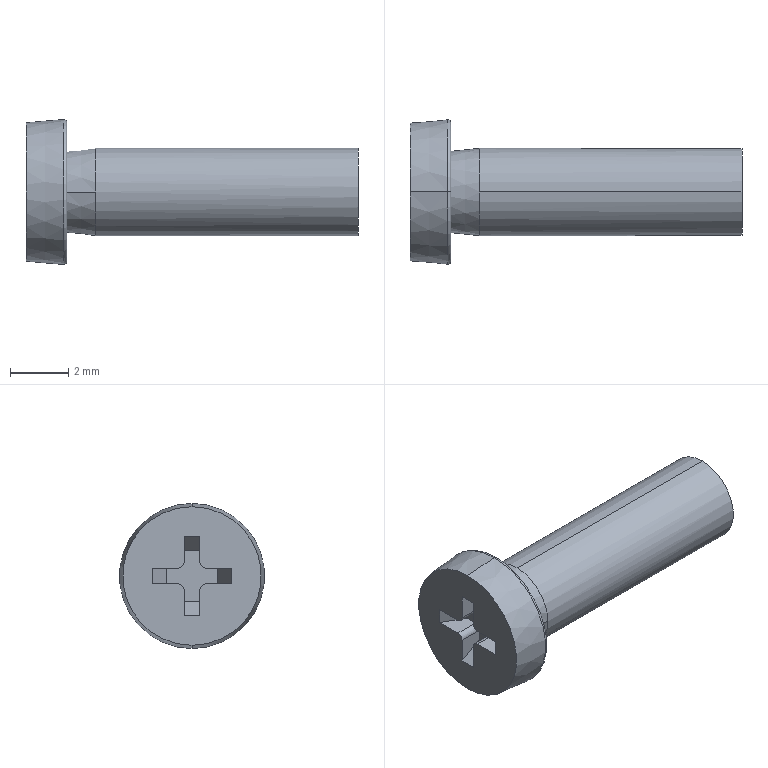Part | SolidWorks | features Draft 2, Fillet 2, Boss 1, Cut 1, Extrusion 1, LPattern 1, PLine 1, RevCut 1 | 1 solid | 28 faces | box 11.4 x 4.982 x 4.982 mm | volume 94.532 mm3 | plane 16 | cylinder 6 | cone 4 | torus 2 | commonest cylinder face diameters 0.4 x4 3 x2
STEP:
#1=CARTESIAN_POINT('',(1.291,0.,2.49));
#2=VERTEX_POINT('',#1);
#3=CARTESIAN_POINT('',(1.291,0.,-2.49));
#4=VERTEX_POINT('',#3);
#5=CARTESIAN_POINT('',(1.291,0.,0.));
#6=DIRECTION('',(-1.,0.,0.));
#7=DIRECTION('',(0.,0.,1.));
#8=AXIS2_PLACEMENT_3D('',#5,#6,#7);
#9=CIRCLE('',#8,2.49);
#10=EDGE_CURVE('',#2,#4,#9,.T.);
#11=ORIENTED_EDGE('',*,*,#10,.F.);
#12=CARTESIAN_POINT('',(1.4,0.,2.391));
#13=VERTEX_POINT('',#12);
#14=CARTESIAN_POINT('',(1.3,0.,2.391));
#15=DIRECTION('',(0.,1.,0.));
#16=DIRECTION('',(0.,0.,1.));
#17=AXIS2_PLACEMENT_3D('',#14,#15,#16);
#18=CIRCLE('',#17,0.1);
#19=EDGE_CURVE('',#2,#13,#18,.T.);
#20=ORIENTED_EDGE('',*,*,#19,.T.);
#21=CARTESIAN_POINT('',(1.4,0.,-2.391));
#22=VERTEX_POINT('',#21);
#23=CARTESIAN_POINT('',(1.4,0.,0.));
#24=DIRECTION('',(1.,0.,0.));
#25=DIRECTION('',(0.,0.,-1.));
#26=AXIS2_PLACEMENT_3D('',#23,#24,#25);
#27=CIRCLE('',#26,2.391);
#28=EDGE_CURVE('',#22,#13,#27,.T.);
#29=ORIENTED_EDGE('',*,*,#28,.F.);
#30=CARTESIAN_POINT('',(1.3,0.,-2.391));
#31=DIRECTION('',(0.,-1.,0.));
#32=DIRECTION('',(1.,0.,0.));
#33=AXIS2_PLACEMENT_3D('',#30,#31,#32);
#34=CIRCLE('',#33,0.1);
#35=EDGE_CURVE('',#4,#22,#34,.T.);
#36=ORIENTED_EDGE('',*,*,#35,.F.);
#37=EDGE_LOOP('',(#11,#20,#29,#36));
#38=FACE_OUTER_BOUND('',#37,.T.);
#39=CARTESIAN_POINT('',(1.3,0.,0.));
#40=DIRECTION('',(1.,0.,0.));
#41=DIRECTION('',(0.,0.,-1.));
#42=AXIS2_PLACEMENT_3D('',#39,#40,#41);
#43=TOROIDAL_SURFACE('',#42,2.391,0.1);
#44=ADVANCED_FACE('',(#38),#43,.T.);
#45=CARTESIAN_POINT('',(11.4,0.,-1.5));
#46=VERTEX_POINT('',#45);
#47=CARTESIAN_POINT('',(11.4,0.,1.5));
#48=VERTEX_POINT('',#47);
#49=CARTESIAN_POINT('',(11.4,0.,0.));
#50=DIRECTION('',(1.,0.,0.));
#51=DIRECTION('',(0.,0.,-1.));
#52=AXIS2_PLACEMENT_3D('',#49,#50,#51);
#53=CIRCLE('',#52,1.5);
#54=EDGE_CURVE('',#46,#48,#53,.T.);
#55=ORIENTED_EDGE('',*,*,#54,.F.);
#56=CARTESIAN_POINT('',(2.4,0.,-1.5));
#57=VERTEX_POINT('',#56);
#58=CARTESIAN_POINT('',(11.4,0.,-1.5));
#59=DIRECTION('',(-1.,0.,0.));
#60=VECTOR('',#59,1000.);
#61=LINE('',#58,#60);
#62=EDGE_CURVE('',#46,#57,#61,.T.);
#63=ORIENTED_EDGE('',*,*,#62,.T.);
#64=CARTESIAN_POINT('',(2.4,1.5,0.));
#65=VERTEX_POINT('',#64);
#66=CARTESIAN_POINT('',(2.4,0.,0.));
#67=DIRECTION('',(1.,0.,0.));
#68=DIRECTION('',(0.,0.,-1.));
#69=AXIS2_PLACEMENT_3D('',#66,#67,#68);
#70=CIRCLE('',#69,1.5);
#71=EDGE_CURVE('',#57,#65,#70,.T.);
#72=ORIENTED_EDGE('',*,*,#71,.T.);
#73=CARTESIAN_POINT('',(2.4,0.,1.5));
#74=VERTEX_POINT('',#73);
#75=CARTESIAN_POINT('',(2.4,0.,0.));
#76=DIRECTION('',(1.,0.,0.));
#77=DIRECTION('',(0.,0.,-1.));
#78=AXIS2_PLACEMENT_3D('',#75,#76,#77);
#79=CIRCLE('',#78,1.5);
#80=EDGE_CURVE('',#65,#74,#79,.T.);
#81=ORIENTED_EDGE('',*,*,#80,.T.);
#82=CARTESIAN_POINT('',(11.4,0.,1.5));
#83=DIRECTION('',(-1.,0.,0.));
#84=VECTOR('',#83,1000.);
#85=LINE('',#82,#84);
#86=EDGE_CURVE('',#48,#74,#85,.T.);
#87=ORIENTED_EDGE('',*,*,#86,.F.);
#88=EDGE_LOOP('',(#55,#63,#72,#81,#87));
#89=FACE_OUTER_BOUND('',#88,.T.);
#90=CARTESIAN_POINT('',(11.4,0.,0.));
#91=DIRECTION('',(-1.,0.,0.));
#92=DIRECTION('',(0.,0.,1.));
#93=AXIS2_PLACEMENT_3D('',#90,#91,#92);
#94=CYLINDRICAL_SURFACE('',#93,1.5);
#95=ADVANCED_FACE('',(#89),#94,.T.);
#96=CARTESIAN_POINT('',(0.,0.,-2.378));
#97=VERTEX_POINT('',#96);
#98=CARTESIAN_POINT('',(0.,0.,2.378));
#99=VERTEX_POINT('',#98);
#100=CARTESIAN_POINT('',(0.,0.,0.));
#101=DIRECTION('',(1.,0.,0.));
#102=DIRECTION('',(0.,0.,-1.));
#103=AXIS2_PLACEMENT_3D('',#100,#101,#102);
#104=CIRCLE('',#103,2.378);
#105=EDGE_CURVE('',#97,#99,#104,.T.);
#106=ORIENTED_EDGE('',*,*,#105,.T.);
#107=CARTESIAN_POINT('',(1.4,0.,2.5));
#108=DIRECTION('',(0.9962,0.,0.08716));
#109=VECTOR('',#108,1000.);
#110=LINE('',#107,#109);
#111=EDGE_CURVE('',#99,#2,#110,.T.);
#112=ORIENTED_EDGE('',*,*,#111,.T.);
#113=ORIENTED_EDGE('',*,*,#10,.T.);
#114=CARTESIAN_POINT('',(1.4,0.,-2.5));
#115=DIRECTION('',(0.9962,0.,-0.08716));
#116=VECTOR('',#115,1000.);
#117=LINE('',#114,#116);
#118=EDGE_CURVE('',#97,#4,#117,.T.);
#119=ORIENTED_EDGE('',*,*,#118,.F.);
#120=EDGE_LOOP('',(#106,#112,#113,#119));
#121=FACE_OUTER_BOUND('',#120,.T.);
#122=CARTESIAN_POINT('',(1.4,0.,0.));
#123=DIRECTION('',(1.,0.,0.));
#124=DIRECTION('',(0.,0.,-1.));
#125=AXIS2_PLACEMENT_3D('',#122,#123,#124);
#126=CONICAL_SURFACE('',#125,2.5,0.08727);
#127=ADVANCED_FACE('',(#121),#126,.T.);
#128=CARTESIAN_POINT('',(1.4,1.395,0.));
#129=VERTEX_POINT('',#128);
#130=CARTESIAN_POINT('',(1.4,-1.395,0.));
#131=VERTEX_POINT('',#130);
#132=CARTESIAN_POINT('',(1.4,0.,0.));
#133=DIRECTION('',(1.,0.,0.));
#134=DIRECTION('',(0.,0.,-1.));
#135=AXIS2_PLACEMENT_3D('',#132,#133,#134);
#136=CIRCLE('',#135,1.395);
#137=EDGE_CURVE('',#129,#131,#136,.T.);
#138=ORIENTED_EDGE('',*,*,#137,.T.);
#139=CARTESIAN_POINT('',(2.4,-1.5,0.));
#140=VERTEX_POINT('',#139);
#141=CARTESIAN_POINT('',(2.4,-1.5,0.));
#142=DIRECTION('',(0.9945,-0.1045,0.));
#143=VECTOR('',#142,1000.);
#144=LINE('',#141,#143);
#145=EDGE_CURVE('',#131,#140,#144,.T.);
#146=ORIENTED_EDGE('',*,*,#145,.T.);
#147=CARTESIAN_POINT('',(2.4,0.,0.));
#148=DIRECTION('',(1.,0.,0.));
#149=DIRECTION('',(0.,0.,-1.));
#150=AXIS2_PLACEMENT_3D('',#147,#148,#149);
#151=CIRCLE('',#150,1.5);
#152=EDGE_CURVE('',#74,#140,#151,.T.);
#153=ORIENTED_EDGE('',*,*,#152,.F.);
#154=ORIENTED_EDGE('',*,*,#80,.F.);
#155=CARTESIAN_POINT('',(2.4,1.5,0.));
#156=DIRECTION('',(0.9945,0.1045,0.));
#157=VECTOR('',#156,1000.);
#158=LINE('',#155,#157);
#159=EDGE_CURVE('',#129,#65,#158,.T.);
#160=ORIENTED_EDGE('',*,*,#159,.F.);
#161=EDGE_LOOP('',(#138,#146,#153,#154,#160));
#162=FACE_OUTER_BOUND('',#161,.T.);
#163=CARTESIAN_POINT('',(2.4,0.,0.));
#164=DIRECTION('',(1.,0.,0.));
#165=DIRECTION('',(0.,1.,0.));
#166=AXIS2_PLACEMENT_3D('',#163,#164,#165);
#167=CONICAL_SURFACE('',#166,1.5,0.1047);
#168=ADVANCED_FACE('',(#162),#167,.T.);
#169=ORIENTED_EDGE('',*,*,#105,.F.);
#170=CARTESIAN_POINT('',(0.,0.,0.));
#171=DIRECTION('',(1.,0.,0.));
#172=DIRECTION('',(0.,0.,-1.));
#173=AXIS2_PLACEMENT_3D('',#170,#171,#172);
#174=CIRCLE('',#173,2.378);
#175=EDGE_CURVE('',#99,#97,#174,.T.);
#176=ORIENTED_EDGE('',*,*,#175,.F.);
#177=EDGE_LOOP('',(#169,#176));
#178=FACE_OUTER_BOUND('',#177,.T.);
#179=CARTESIAN_POINT('',(0.,0.27,-1.35));
#180=VERTEX_POINT('',#179);
#181=CARTESIAN_POINT('',(0.,0.27,-0.47));
#182=VERTEX_POINT('',#181);
#183=CARTESIAN_POINT('',(0.,0.27,-0.27));
#184=DIRECTION('',(0.,0.,1.));
#185=VECTOR('',#184,1000.);
#186=LINE('',#183,#185);
#187=EDGE_CURVE('',#180,#182,#186,.T.);
#188=ORIENTED_EDGE('',*,*,#187,.T.);
#189=CARTESIAN_POINT('',(0.,0.47,-0.27));
#190=VERTEX_POINT('',#189);
#191=CARTESIAN_POINT('',(0.,0.47,-0.47));
#192=DIRECTION('',(-1.,0.,0.));
#193=DIRECTION('',(0.,0.,-1.));
#194=AXIS2_PLACEMENT_3D('',#191,#192,#193);
#195=CIRCLE('',#194,0.2);
#196=EDGE_CURVE('',#182,#190,#195,.T.);
#197=ORIENTED_EDGE('',*,*,#196,.T.);
#198=CARTESIAN_POINT('',(0.,1.35,-0.27));
#199=VERTEX_POINT('',#198);
#200=CARTESIAN_POINT('',(0.,1.35,-0.27));
#201=DIRECTION('',(0.,1.,0.));
#202=VECTOR('',#201,1000.);
#203=LINE('',#200,#202);
#204=EDGE_CURVE('',#190,#199,#203,.T.);
#205=ORIENTED_EDGE('',*,*,#204,.T.);
#206=CARTESIAN_POINT('',(0.,1.35,0.27));
#207=VERTEX_POINT('',#206);
#208=CARTESIAN_POINT('',(0.,1.35,0.27));
#209=DIRECTION('',(0.,0.,1.));
#210=VECTOR('',#209,1000.);
#211=LINE('',#208,#210);
#212=EDGE_CURVE('',#199,#207,#211,.T.);
#213=ORIENTED_EDGE('',*,*,#212,.T.);
#214=CARTESIAN_POINT('',(0.,0.47,0.27));
#215=VERTEX_POINT('',#214);
#216=CARTESIAN_POINT('',(0.,1.35,0.27));
#217=DIRECTION('',(0.,-1.,0.));
#218=VECTOR('',#217,1000.);
#219=LINE('',#216,#218);
#220=EDGE_CURVE('',#207,#215,#219,.T.);
#221=ORIENTED_EDGE('',*,*,#220,.T.);
#222=CARTESIAN_POINT('',(0.,0.27,0.47));
#223=VERTEX_POINT('',#222);
#224=CARTESIAN_POINT('',(0.,0.47,0.47));
#225=DIRECTION('',(-1.,0.,0.));
#226=DIRECTION('',(0.,0.,-1.));
#227=AXIS2_PLACEMENT_3D('',#224,#225,#226);
#228=CIRCLE('',#227,0.2);
#229=EDGE_CURVE('',#215,#223,#228,.T.);
#230=ORIENTED_EDGE('',*,*,#229,.T.);
#231=CARTESIAN_POINT('',(0.,0.27,1.35));
#232=VERTEX_POINT('',#231);
#233=CARTESIAN_POINT('',(0.,0.27,1.35));
#234=DIRECTION('',(0.,0.,1.));
#235=VECTOR('',#234,1000.);
#236=LINE('',#233,#235);
#237=EDGE_CURVE('',#223,#232,#236,.T.);
#238=ORIENTED_EDGE('',*,*,#237,.T.);
#239=CARTESIAN_POINT('',(0.,-0.27,1.35));
#240=VERTEX_POINT('',#239);
#241=CARTESIAN_POINT('',(0.,0.27,1.35));
#242=DIRECTION('',(0.,-1.,0.));
#243=VECTOR('',#242,1000.);
#244=LINE('',#241,#243);
#245=EDGE_CURVE('',#232,#240,#244,.T.);
#246=ORIENTED_EDGE('',*,*,#245,.T.);
#247=CARTESIAN_POINT('',(0.,-0.27,0.47));
#248=VERTEX_POINT('',#247);
#249=CARTESIAN_POINT('',(0.,-0.27,1.35));
#250=DIRECTION('',(0.,0.,-1.));
#251=VECTOR('',#250,1000.);
#252=LINE('',#249,#251);
#253=EDGE_CURVE('',#240,#248,#252,.T.);
#254=ORIENTED_EDGE('',*,*,#253,.T.);
#255=CARTESIAN_POINT('',(0.,-0.47,0.27));
#256=VERTEX_POINT('',#255);
#257=CARTESIAN_POINT('',(0.,-0.47,0.47));
#258=DIRECTION('',(-1.,0.,0.));
#259=DIRECTION('',(0.,0.,-1.));
#260=AXIS2_PLACEMENT_3D('',#257,#258,#259);
#261=CIRCLE('',#260,0.2);
#262=EDGE_CURVE('',#248,#256,#261,.T.);
#263=ORIENTED_EDGE('',*,*,#262,.T.);
#264=CARTESIAN_POINT('',(0.,-1.35,0.27));
#265=VERTEX_POINT('',#264);
#266=CARTESIAN_POINT('',(0.,-0.27,0.27));
#267=DIRECTION('',(0.,-1.,0.));
#268=VECTOR('',#267,1000.);
#269=LINE('',#266,#268);
#270=EDGE_CURVE('',#256,#265,#269,.T.);
#271=ORIENTED_EDGE('',*,*,#270,.T.);
#272=CARTESIAN_POINT('',(0.,-1.35,-0.27));
#273=VERTEX_POINT('',#272);
#274=CARTESIAN_POINT('',(0.,-1.35,0.27));
#275=DIRECTION('',(0.,0.,-1.));
#276=VECTOR('',#275,1000.);
#277=LINE('',#274,#276);
#278=EDGE_CURVE('',#265,#273,#277,.T.);
#279=ORIENTED_EDGE('',*,*,#278,.T.);
#280=CARTESIAN_POINT('',(0.,-0.47,-0.27));
#281=VERTEX_POINT('',#280);
#282=CARTESIAN_POINT('',(0.,-0.27,-0.27));
#283=DIRECTION('',(0.,1.,0.));
#284=VECTOR('',#283,1000.);
#285=LINE('',#282,#284);
#286=EDGE_CURVE('',#273,#281,#285,.T.);
#287=ORIENTED_EDGE('',*,*,#286,.T.);
#288=CARTESIAN_POINT('',(0.,-0.27,-0.47));
#289=VERTEX_POINT('',#288);
#290=CARTESIAN_POINT('',(0.,-0.47,-0.47));
#291=DIRECTION('',(-1.,0.,0.));
#292=DIRECTION('',(0.,0.,-1.));
#293=AXIS2_PLACEMENT_3D('',#290,#291,#292);
#294=CIRCLE('',#293,0.2);
#295=EDGE_CURVE('',#281,#289,#294,.T.);
#296=ORIENTED_EDGE('',*,*,#295,.T.);
#297=CARTESIAN_POINT('',(0.,-0.27,-1.35));
#298=VERTEX_POINT('',#297);
#299=CARTESIAN_POINT('',(0.,-0.27,-0.27));
#300=DIRECTION('',(0.,0.,-1.));
#301=VECTOR('',#300,1000.);
#302=LINE('',#299,#301);
#303=EDGE_CURVE('',#289,#298,#302,.T.);
#304=ORIENTED_EDGE('',*,*,#303,.T.);
#305=CARTESIAN_POINT('',(0.,0.27,-1.35));
#306=DIRECTION('',(0.,1.,0.));
#307=VECTOR('',#306,1000.);
#308=LINE('',#305,#307);
#309=EDGE_CURVE('',#298,#180,#308,.T.);
#310=ORIENTED_EDGE('',*,*,#309,.T.);
#311=EDGE_LOOP('',(#188,#197,#205,#213,#221,#230,#238,#246,#254,#263,#271,#279,#287,#296,#304,#310));
#312=FACE_BOUND('',#311,.T.);
#313=CARTESIAN_POINT('',(0.,0.,0.));
#314=DIRECTION('',(1.,0.,0.));
#315=DIRECTION('',(0.,0.,-1.));
#316=AXIS2_PLACEMENT_3D('',#313,#314,#315);
#317=PLANE('',#316);
#318=ADVANCED_FACE('',(#178,#312),#317,.F.);
#319=ORIENTED_EDGE('',*,*,#145,.F.);
#320=CARTESIAN_POINT('',(1.4,0.,0.));
#321=DIRECTION('',(1.,0.,0.));
#322=DIRECTION('',(0.,0.,-1.));
#323=AXIS2_PLACEMENT_3D('',#320,#321,#322);
#324=CIRCLE('',#323,1.395);
#325=EDGE_CURVE('',#131,#129,#324,.T.);
#326=ORIENTED_EDGE('',*,*,#325,.T.);
#327=ORIENTED_EDGE('',*,*,#159,.T.);
#328=ORIENTED_EDGE('',*,*,#71,.F.);
#329=CARTESIAN_POINT('',(2.4,0.,0.));
#330=DIRECTION('',(1.,0.,0.));
#331=DIRECTION('',(0.,0.,-1.));
#332=AXIS2_PLACEMENT_3D('',#329,#330,#331);
#333=CIRCLE('',#332,1.5);
#334=EDGE_CURVE('',#140,#57,#333,.T.);
#335=ORIENTED_EDGE('',*,*,#334,.F.);
#336=EDGE_LOOP('',(#319,#326,#327,#328,#335));
#337=FACE_OUTER_BOUND('',#336,.T.);
#338=CARTESIAN_POINT('',(2.4,0.,0.));
#339=DIRECTION('',(1.,0.,0.));
#340=DIRECTION('',(0.,1.,0.));
#341=AXIS2_PLACEMENT_3D('',#338,#339,#340);
#342=CONICAL_SURFACE('',#341,1.5,0.1047);
#343=ADVANCED_FACE('',(#337),#342,.T.);
#344=ORIENTED_EDGE('',*,*,#28,.T.);
#345=CARTESIAN_POINT('',(1.4,0.,0.));
#346=DIRECTION('',(1.,0.,0.));
#347=DIRECTION('',(0.,0.,-1.));
#348=AXIS2_PLACEMENT_3D('',#345,#346,#347);
#349=CIRCLE('',#348,2.391);
#350=EDGE_CURVE('',#13,#22,#349,.T.);
#351=ORIENTED_EDGE('',*,*,#350,.T.);
#352=EDGE_LOOP('',(#344,#351));
#353=FACE_OUTER_BOUND('',#352,.T.);
#354=ORIENTED_EDGE('',*,*,#137,.F.);
#355=ORIENTED_EDGE('',*,*,#325,.F.);
#356=EDGE_LOOP('',(#354,#355));
#357=FACE_BOUND('',#356,.T.);
#358=CARTESIAN_POINT('',(1.4,0.,0.));
#359=DIRECTION('',(1.,0.,0.));
#360=DIRECTION('',(0.,0.,-1.));
#361=AXIS2_PLACEMENT_3D('',#358,#359,#360);
#362=PLANE('',#361);
#363=ADVANCED_FACE('',(#353,#357),#362,.T.);
#364=ORIENTED_EDGE('',*,*,#111,.F.);
#365=ORIENTED_EDGE('',*,*,#175,.T.);
#366=ORIENTED_EDGE('',*,*,#118,.T.);
#367=CARTESIAN_POINT('',(1.291,0.,0.));
#368=DIRECTION('',(-1.,0.,0.));
#369=DIRECTION('',(0.,0.,1.));
#370=AXIS2_PLACEMENT_3D('',#367,#368,#369);
#371=CIRCLE('',#370,2.49);
#372=EDGE_CURVE('',#4,#2,#371,.T.);
#373=ORIENTED_EDGE('',*,*,#372,.T.);
#374=EDGE_LOOP('',(#364,#365,#366,#373));
#375=FACE_OUTER_BOUND('',#374,.T.);
#376=CARTESIAN_POINT('',(1.4,0.,0.));
#377=DIRECTION('',(1.,0.,0.));
#378=DIRECTION('',(0.,0.,-1.));
#379=AXIS2_PLACEMENT_3D('',#376,#377,#378);
#380=CONICAL_SURFACE('',#379,2.5,0.08727);
#381=ADVANCED_FACE('',(#375),#380,.T.);
#382=ORIENTED_EDGE('',*,*,#62,.F.);
#383=CARTESIAN_POINT('',(11.4,0.,0.));
#384=DIRECTION('',(1.,0.,0.));
#385=DIRECTION('',(0.,0.,-1.));
#386=AXIS2_PLACEMENT_3D('',#383,#384,#385);
#387=CIRCLE('',#386,1.5);
#388=EDGE_CURVE('',#48,#46,#387,.T.);
#389=ORIENTED_EDGE('',*,*,#388,.F.);
#390=ORIENTED_EDGE('',*,*,#86,.T.);
#391=ORIENTED_EDGE('',*,*,#152,.T.);
#392=ORIENTED_EDGE('',*,*,#334,.T.);
#393=EDGE_LOOP('',(#382,#389,#390,#391,#392));
#394=FACE_OUTER_BOUND('',#393,.T.);
#395=CARTESIAN_POINT('',(11.4,0.,0.));
#396=DIRECTION('',(-1.,0.,0.));
#397=DIRECTION('',(0.,0.,1.));
#398=AXIS2_PLACEMENT_3D('',#395,#396,#397);
#399=CYLINDRICAL_SURFACE('',#398,1.5);
#400=ADVANCED_FACE('',(#394),#399,.T.);
#401=ORIENTED_EDGE('',*,*,#388,.T.);
#402=ORIENTED_EDGE('',*,*,#54,.T.);
#403=EDGE_LOOP('',(#401,#402));
#404=FACE_OUTER_BOUND('',#403,.T.);
#405=CARTESIAN_POINT('',(11.4,0.,0.));
#406=DIRECTION('',(1.,0.,0.));
#407=DIRECTION('',(0.,0.,-1.));
#408=AXIS2_PLACEMENT_3D('',#405,#406,#407);
#409=PLANE('',#408);
#410=ADVANCED_FACE('',(#404),#409,.T.);
#411=CARTESIAN_POINT('',(0.84,0.865,0.27));
#412=VERTEX_POINT('',#411);
#413=CARTESIAN_POINT('',(0.84,0.47,0.27));
#414=VERTEX_POINT('',#413);
#415=CARTESIAN_POINT('',(0.84,1.35,0.27));
#416=DIRECTION('',(0.,-1.,0.));
#417=VECTOR('',#416,1000.);
#418=LINE('',#415,#417);
#419=EDGE_CURVE('',#412,#414,#418,.T.);
#420=ORIENTED_EDGE('',*,*,#419,.T.);
#421=CARTESIAN_POINT('',(0.84,0.47,0.27));
#422=DIRECTION('',(-1.,0.,0.));
#423=VECTOR('',#422,1000.);
#424=LINE('',#421,#423);
#425=EDGE_CURVE('',#414,#215,#424,.T.);
#426=ORIENTED_EDGE('',*,*,#425,.T.);
#427=ORIENTED_EDGE('',*,*,#220,.F.);
#428=CARTESIAN_POINT('',(0.63,0.9863,0.27));
#429=DIRECTION('',(-0.866,0.5,0.));
#430=VECTOR('',#429,1000.);
#431=LINE('',#428,#430);
#432=EDGE_CURVE('',#412,#207,#431,.T.);
#433=ORIENTED_EDGE('',*,*,#432,.F.);
#434=EDGE_LOOP('',(#420,#426,#427,#433));
#435=FACE_OUTER_BOUND('',#434,.T.);
#436=CARTESIAN_POINT('',(0.84,1.35,0.27));
#437=DIRECTION('',(0.,0.,-1.));
#438=DIRECTION('',(0.,1.,0.));
#439=AXIS2_PLACEMENT_3D('',#436,#437,#438);
#440=PLANE('',#439);
#441=ADVANCED_FACE('',(#435),#440,.T.);
#442=ORIENTED_EDGE('',*,*,#237,.F.);
#443=CARTESIAN_POINT('',(0.84,0.27,0.47));
#444=VERTEX_POINT('',#443);
#445=CARTESIAN_POINT('',(0.84,0.27,0.47));
#446=DIRECTION('',(1.,0.,0.));
#447=VECTOR('',#446,1000.);
#448=LINE('',#445,#447);
#449=EDGE_CURVE('',#223,#444,#448,.T.);
#450=ORIENTED_EDGE('',*,*,#449,.T.);
#451=CARTESIAN_POINT('',(0.84,0.27,0.865));
#452=VERTEX_POINT('',#451);
#453=CARTESIAN_POINT('',(0.84,0.27,1.35));
#454=DIRECTION('',(0.,0.,1.));
#455=VECTOR('',#454,1000.);
#456=LINE('',#453,#455);
#457=EDGE_CURVE('',#444,#452,#456,.T.);
#458=ORIENTED_EDGE('',*,*,#457,.T.);
#459=CARTESIAN_POINT('',(0.,0.27,1.35));
#460=DIRECTION('',(-0.866,0.,0.5));
#461=VECTOR('',#460,1000.);
#462=LINE('',#459,#461);
#463=EDGE_CURVE('',#452,#232,#462,.T.);
#464=ORIENTED_EDGE('',*,*,#463,.T.);
#465=EDGE_LOOP('',(#442,#450,#458,#464));
#466=FACE_OUTER_BOUND('',#465,.T.);
#467=CARTESIAN_POINT('',(0.84,0.27,1.35));
#468=DIRECTION('',(0.,-1.,0.));
#469=DIRECTION('',(0.,0.,-1.));
#470=AXIS2_PLACEMENT_3D('',#467,#468,#469);
#471=PLANE('',#470);
#472=ADVANCED_FACE('',(#466),#471,.T.);
#473=ORIENTED_EDGE('',*,*,#245,.F.);
#474=ORIENTED_EDGE('',*,*,#463,.F.);
#475=CARTESIAN_POINT('',(0.84,-0.27,0.865));
#476=VERTEX_POINT('',#475);
#477=CARTESIAN_POINT('',(0.84,0.27,0.865));
#478=DIRECTION('',(0.,-1.,0.));
#479=VECTOR('',#478,1000.);
#480=LINE('',#477,#479);
#481=EDGE_CURVE('',#452,#476,#480,.T.);
#482=ORIENTED_EDGE('',*,*,#481,.T.);
#483=CARTESIAN_POINT('',(0.63,-0.27,0.9863));
#484=DIRECTION('',(-0.866,0.,0.5));
#485=VECTOR('',#484,1000.);
#486=LINE('',#483,#485);
#487=EDGE_CURVE('',#476,#240,#486,.T.);
#488=ORIENTED_EDGE('',*,*,#487,.T.);
#489=EDGE_LOOP('',(#473,#474,#482,#488));
#490=FACE_OUTER_BOUND('',#489,.T.);
#491=CARTESIAN_POINT('',(0.,0.27,1.35));
#492=DIRECTION('',(-0.5,0.,-0.866));
#493=DIRECTION('',(-0.866,0.,0.5));
#494=AXIS2_PLACEMENT_3D('',#491,#492,#493);
#495=PLANE('',#494);
#496=ADVANCED_FACE('',(#490),#495,.T.);
#497=CARTESIAN_POINT('',(0.84,-0.27,0.47));
#498=VERTEX_POINT('',#497);
#499=CARTESIAN_POINT('',(0.84,-0.27,1.35));
#500=DIRECTION('',(0.,0.,-1.));
#501=VECTOR('',#500,1000.);
#502=LINE('',#499,#501);
#503=EDGE_CURVE('',#476,#498,#502,.T.);
#504=ORIENTED_EDGE('',*,*,#503,.T.);
#505=CARTESIAN_POINT('',(0.84,-0.27,0.47));
#506=DIRECTION('',(-1.,0.,0.));
#507=VECTOR('',#506,1000.);
#508=LINE('',#505,#507);
#509=EDGE_CURVE('',#498,#248,#508,.T.);
#510=ORIENTED_EDGE('',*,*,#509,.T.);
#511=ORIENTED_EDGE('',*,*,#253,.F.);
#512=ORIENTED_EDGE('',*,*,#487,.F.);
#513=EDGE_LOOP('',(#504,#510,#511,#512));
#514=FACE_OUTER_BOUND('',#513,.T.);
#515=CARTESIAN_POINT('',(0.84,-0.27,1.35));
#516=DIRECTION('',(0.,1.,0.));
#517=DIRECTION('',(0.,0.,1.));
#518=AXIS2_PLACEMENT_3D('',#515,#516,#517);
#519=PLANE('',#518);
#520=ADVANCED_FACE('',(#514),#519,.T.);
#521=ORIENTED_EDGE('',*,*,#270,.F.);
#522=CARTESIAN_POINT('',(0.84,-0.47,0.27));
#523=VERTEX_POINT('',#522);
#524=CARTESIAN_POINT('',(0.84,-0.47,0.27));
#525=DIRECTION('',(1.,0.,0.));
#526=VECTOR('',#525,1000.);
#527=LINE('',#524,#526);
#528=EDGE_CURVE('',#256,#523,#527,.T.);
#529=ORIENTED_EDGE('',*,*,#528,.T.);
#530=CARTESIAN_POINT('',(0.84,-0.865,0.27));
#531=VERTEX_POINT('',#530);
#532=CARTESIAN_POINT('',(0.84,-0.27,0.27));
#533=DIRECTION('',(0.,-1.,0.));
#534=VECTOR('',#533,1000.);
#535=LINE('',#532,#534);
#536=EDGE_CURVE('',#523,#531,#535,.T.);
#537=ORIENTED_EDGE('',*,*,#536,.T.);
#538=CARTESIAN_POINT('',(0.,-1.35,0.27));
#539=DIRECTION('',(-0.866,-0.5,0.));
#540=VECTOR('',#539,1000.);
#541=LINE('',#538,#540);
#542=EDGE_CURVE('',#531,#265,#541,.T.);
#543=ORIENTED_EDGE('',*,*,#542,.T.);
#544=EDGE_LOOP('',(#521,#529,#537,#543));
#545=FACE_OUTER_BOUND('',#544,.T.);
#546=CARTESIAN_POINT('',(0.84,-0.27,0.27));
#547=DIRECTION('',(0.,0.,-1.));
#548=DIRECTION('',(0.,1.,0.));
#549=AXIS2_PLACEMENT_3D('',#546,#547,#548);
#550=PLANE('',#549);
#551=ADVANCED_FACE('',(#545),#550,.T.);
#552=ORIENTED_EDGE('',*,*,#278,.F.);
#553=ORIENTED_EDGE('',*,*,#542,.F.);
#554=CARTESIAN_POINT('',(0.84,-0.865,-0.27));
#555=VERTEX_POINT('',#554);
#556=CARTESIAN_POINT('',(0.84,-0.865,0.27));
#557=DIRECTION('',(0.,0.,-1.));
#558=VECTOR('',#557,1000.);
#559=LINE('',#556,#558);
#560=EDGE_CURVE('',#531,#555,#559,.T.);
#561=ORIENTED_EDGE('',*,*,#560,.T.);
#562=CARTESIAN_POINT('',(1.098,-0.7163,-0.27));
#563=DIRECTION('',(-0.866,-0.5,0.));
#564=VECTOR('',#563,1000.);
#565=LINE('',#562,#564);
#566=EDGE_CURVE('',#555,#273,#565,.T.);
#567=ORIENTED_EDGE('',*,*,#566,.T.);
#568=EDGE_LOOP('',(#552,#553,#561,#567));
#569=FACE_OUTER_BOUND('',#568,.T.);
#570=CARTESIAN_POINT('',(0.,-1.35,0.27));
#571=DIRECTION('',(-0.5,0.866,0.));
#572=DIRECTION('',(-0.866,-0.5,0.));
#573=AXIS2_PLACEMENT_3D('',#570,#571,#572);
#574=PLANE('',#573);
#575=ADVANCED_FACE('',(#569),#574,.T.);
#576=CARTESIAN_POINT('',(0.84,-0.47,-0.27));
#577=VERTEX_POINT('',#576);
#578=CARTESIAN_POINT('',(0.84,-0.27,-0.27));
#579=DIRECTION('',(0.,1.,0.));
#580=VECTOR('',#579,1000.);
#581=LINE('',#578,#580);
#582=EDGE_CURVE('',#555,#577,#581,.T.);
#583=ORIENTED_EDGE('',*,*,#582,.T.);
#584=CARTESIAN_POINT('',(0.84,-0.47,-0.27));
#585=DIRECTION('',(-1.,0.,0.));
#586=VECTOR('',#585,1000.);
#587=LINE('',#584,#586);
#588=EDGE_CURVE('',#577,#281,#587,.T.);
#589=ORIENTED_EDGE('',*,*,#588,.T.);
#590=ORIENTED_EDGE('',*,*,#286,.F.);
#591=ORIENTED_EDGE('',*,*,#566,.F.);
#592=EDGE_LOOP('',(#583,#589,#590,#591));
#593=FACE_OUTER_BOUND('',#592,.T.);
#594=CARTESIAN_POINT('',(0.84,-0.27,-0.27));
#595=DIRECTION('',(0.,0.,1.));
#596=DIRECTION('',(0.,-1.,0.));
#597=AXIS2_PLACEMENT_3D('',#594,#595,#596);
#598=PLANE('',#597);
#599=ADVANCED_FACE('',(#593),#598,.T.);
#600=ORIENTED_EDGE('',*,*,#303,.F.);
#601=CARTESIAN_POINT('',(0.84,-0.27,-0.47));
#602=VERTEX_POINT('',#601);
#603=CARTESIAN_POINT('',(0.84,-0.27,-0.47));
#604=DIRECTION('',(1.,0.,0.));
#605=VECTOR('',#604,1000.);
#606=LINE('',#603,#605);
#607=EDGE_CURVE('',#289,#602,#606,.T.);
#608=ORIENTED_EDGE('',*,*,#607,.T.);
#609=CARTESIAN_POINT('',(0.84,-0.27,-0.865));
#610=VERTEX_POINT('',#609);
#611=CARTESIAN_POINT('',(0.84,-0.27,-0.27));
#612=DIRECTION('',(0.,0.,-1.));
#613=VECTOR('',#612,1000.);
#614=LINE('',#611,#613);
#615=EDGE_CURVE('',#602,#610,#614,.T.);
#616=ORIENTED_EDGE('',*,*,#615,.T.);
#617=CARTESIAN_POINT('',(0.,-0.27,-1.35));
#618=DIRECTION('',(-0.866,0.,-0.5));
#619=VECTOR('',#618,1000.);
#620=LINE('',#617,#619);
#621=EDGE_CURVE('',#610,#298,#620,.T.);
#622=ORIENTED_EDGE('',*,*,#621,.T.);
#623=EDGE_LOOP('',(#600,#608,#616,#622));
#624=FACE_OUTER_BOUND('',#623,.T.);
#625=CARTESIAN_POINT('',(0.84,-0.27,-0.27));
#626=DIRECTION('',(0.,1.,0.));
#627=DIRECTION('',(0.,0.,1.));
#628=AXIS2_PLACEMENT_3D('',#625,#626,#627);
#629=PLANE('',#628);
#630=ADVANCED_FACE('',(#624),#629,.T.);
#631=ORIENTED_EDGE('',*,*,#309,.F.);
#632=ORIENTED_EDGE('',*,*,#621,.F.);
#633=CARTESIAN_POINT('',(0.84,0.27,-0.865));
#634=VERTEX_POINT('',#633);
#635=CARTESIAN_POINT('',(0.84,0.27,-0.865));
#636=DIRECTION('',(0.,1.,0.));
#637=VECTOR('',#636,1000.);
#638=LINE('',#635,#637);
#639=EDGE_CURVE('',#610,#634,#638,.T.);
#640=ORIENTED_EDGE('',*,*,#639,.T.);
#641=CARTESIAN_POINT('',(1.098,0.27,-0.7163));
#642=DIRECTION('',(-0.866,0.,-0.5));
#643=VECTOR('',#642,1000.);
#644=LINE('',#641,#643);
#645=EDGE_CURVE('',#634,#180,#644,.T.);
#646=ORIENTED_EDGE('',*,*,#645,.T.);
#647=EDGE_LOOP('',(#631,#632,#640,#646));
#648=FACE_OUTER_BOUND('',#647,.T.);
#649=CARTESIAN_POINT('',(0.,0.27,-1.35));
#650=DIRECTION('',(-0.5,0.,0.866));
#651=DIRECTION('',(0.866,0.,0.5));
#652=AXIS2_PLACEMENT_3D('',#649,#650,#651);
#653=PLANE('',#652);
#654=ADVANCED_FACE('',(#648),#653,.T.);
#655=CARTESIAN_POINT('',(0.84,0.27,-0.47));
#656=VERTEX_POINT('',#655);
#657=CARTESIAN_POINT('',(0.84,0.27,-0.27));
#658=DIRECTION('',(0.,0.,1.));
#659=VECTOR('',#658,1000.);
#660=LINE('',#657,#659);
#661=EDGE_CURVE('',#634,#656,#660,.T.);
#662=ORIENTED_EDGE('',*,*,#661,.T.);
#663=CARTESIAN_POINT('',(0.84,0.27,-0.47));
#664=DIRECTION('',(-1.,0.,0.));
#665=VECTOR('',#664,1000.);
#666=LINE('',#663,#665);
#667=EDGE_CURVE('',#656,#182,#666,.T.);
#668=ORIENTED_EDGE('',*,*,#667,.T.);
#669=ORIENTED_EDGE('',*,*,#187,.F.);
#670=ORIENTED_EDGE('',*,*,#645,.F.);
#671=EDGE_LOOP('',(#662,#668,#669,#670));
#672=FACE_OUTER_BOUND('',#671,.T.);
#673=CARTESIAN_POINT('',(0.84,0.27,-0.27));
#674=DIRECTION('',(0.,-1.,0.));
#675=DIRECTION('',(0.,0.,-1.));
#676=AXIS2_PLACEMENT_3D('',#673,#674,#675);
#677=PLANE('',#676);
#678=ADVANCED_FACE('',(#672),#677,.T.);
#679=ORIENTED_EDGE('',*,*,#204,.F.);
#680=CARTESIAN_POINT('',(0.84,0.47,-0.27));
#681=VERTEX_POINT('',#680);
#682=CARTESIAN_POINT('',(0.84,0.47,-0.27));
#683=DIRECTION('',(1.,0.,0.));
#684=VECTOR('',#683,1000.);
#685=LINE('',#682,#684);
#686=EDGE_CURVE('',#190,#681,#685,.T.);
#687=ORIENTED_EDGE('',*,*,#686,.T.);
#688=CARTESIAN_POINT('',(0.84,0.865,-0.27));
#689=VERTEX_POINT('',#688);
#690=CARTESIAN_POINT('',(0.84,1.35,-0.27));
#691=DIRECTION('',(0.,1.,0.));
#692=VECTOR('',#691,1000.);
#693=LINE('',#690,#692);
#694=EDGE_CURVE('',#681,#689,#693,.T.);
#695=ORIENTED_EDGE('',*,*,#694,.T.);
#696=CARTESIAN_POINT('',(0.,1.35,-0.27));
#697=DIRECTION('',(-0.866,0.5,0.));
#698=VECTOR('',#697,1000.);
#699=LINE('',#696,#698);
#700=EDGE_CURVE('',#689,#199,#699,.T.);
#701=ORIENTED_EDGE('',*,*,#700,.T.);
#702=EDGE_LOOP('',(#679,#687,#695,#701));
#703=FACE_OUTER_BOUND('',#702,.T.);
#704=CARTESIAN_POINT('',(0.84,1.35,-0.27));
#705=DIRECTION('',(0.,0.,1.));
#706=DIRECTION('',(0.,-1.,0.));
#707=AXIS2_PLACEMENT_3D('',#704,#705,#706);
#708=PLANE('',#707);
#709=ADVANCED_FACE('',(#703),#708,.T.);
#710=ORIENTED_EDGE('',*,*,#212,.F.);
#711=ORIENTED_EDGE('',*,*,#700,.F.);
#712=CARTESIAN_POINT('',(0.84,0.865,0.27));
#713=DIRECTION('',(0.,0.,1.));
#714=VECTOR('',#713,1000.);
#715=LINE('',#712,#714);
#716=EDGE_CURVE('',#689,#412,#715,.T.);
#717=ORIENTED_EDGE('',*,*,#716,.T.);
#718=ORIENTED_EDGE('',*,*,#432,.T.);
#719=EDGE_LOOP('',(#710,#711,#717,#718));
#720=FACE_OUTER_BOUND('',#719,.T.);
#721=CARTESIAN_POINT('',(0.,1.35,0.27));
#722=DIRECTION('',(-0.5,-0.866,0.));
#723=DIRECTION('',(0.866,-0.5,0.));
#724=AXIS2_PLACEMENT_3D('',#721,#722,#723);
#725=PLANE('',#724);
#726=ADVANCED_FACE('',(#720),#725,.T.);
#727=ORIENTED_EDGE('',*,*,#419,.F.);
#728=ORIENTED_EDGE('',*,*,#716,.F.);
#729=ORIENTED_EDGE('',*,*,#694,.F.);
#730=CARTESIAN_POINT('',(0.84,0.47,-0.47));
#731=DIRECTION('',(1.,0.,0.));
#732=DIRECTION('',(0.,0.,-1.));
#733=AXIS2_PLACEMENT_3D('',#730,#731,#732);
#734=CIRCLE('',#733,0.2);
#735=EDGE_CURVE('',#681,#656,#734,.T.);
#736=ORIENTED_EDGE('',*,*,#735,.T.);
#737=ORIENTED_EDGE('',*,*,#661,.F.);
#738=ORIENTED_EDGE('',*,*,#639,.F.);
#739=ORIENTED_EDGE('',*,*,#615,.F.);
#740=CARTESIAN_POINT('',(0.84,-0.47,-0.47));
#741=DIRECTION('',(1.,0.,0.));
#742=DIRECTION('',(0.,0.,-1.));
#743=AXIS2_PLACEMENT_3D('',#740,#741,#742);
#744=CIRCLE('',#743,0.2);
#745=EDGE_CURVE('',#602,#577,#744,.T.);
#746=ORIENTED_EDGE('',*,*,#745,.T.);
#747=ORIENTED_EDGE('',*,*,#582,.F.);
#748=ORIENTED_EDGE('',*,*,#560,.F.);
#749=ORIENTED_EDGE('',*,*,#536,.F.);
#750=CARTESIAN_POINT('',(0.84,-0.47,0.47));
#751=DIRECTION('',(1.,0.,0.));
#752=DIRECTION('',(0.,0.,-1.));
#753=AXIS2_PLACEMENT_3D('',#750,#751,#752);
#754=CIRCLE('',#753,0.2);
#755=EDGE_CURVE('',#523,#498,#754,.T.);
#756=ORIENTED_EDGE('',*,*,#755,.T.);
#757=ORIENTED_EDGE('',*,*,#503,.F.);
#758=ORIENTED_EDGE('',*,*,#481,.F.);
#759=ORIENTED_EDGE('',*,*,#457,.F.);
#760=CARTESIAN_POINT('',(0.84,0.47,0.47));
#761=DIRECTION('',(1.,0.,0.));
#762=DIRECTION('',(0.,0.,-1.));
#763=AXIS2_PLACEMENT_3D('',#760,#761,#762);
#764=CIRCLE('',#763,0.2);
#765=EDGE_CURVE('',#444,#414,#764,.T.);
#766=ORIENTED_EDGE('',*,*,#765,.T.);
#767=EDGE_LOOP('',(#727,#728,#729,#736,#737,#738,#739,#746,#747,#748,#749,#756,#757,#758,#759,#766));
#768=FACE_OUTER_BOUND('',#767,.T.);
#769=CARTESIAN_POINT('',(0.84,-0.27,0.27));
#770=DIRECTION('',(1.,0.,0.));
#771=DIRECTION('',(0.,0.,-1.));
#772=AXIS2_PLACEMENT_3D('',#769,#770,#771);
#773=PLANE('',#772);
#774=ADVANCED_FACE('',(#768),#773,.F.);
#775=ORIENTED_EDGE('',*,*,#735,.F.);
#776=ORIENTED_EDGE('',*,*,#686,.F.);
#777=ORIENTED_EDGE('',*,*,#196,.F.);
#778=ORIENTED_EDGE('',*,*,#667,.F.);
#779=EDGE_LOOP('',(#775,#776,#777,#778));
#780=FACE_OUTER_BOUND('',#779,.T.);
#781=CARTESIAN_POINT('',(0.84,0.47,-0.47));
#782=DIRECTION('',(-1.,0.,0.));
#783=DIRECTION('',(0.,0.,1.));
#784=AXIS2_PLACEMENT_3D('',#781,#782,#783);
#785=CYLINDRICAL_SURFACE('',#784,0.2);
#786=ADVANCED_FACE('',(#780),#785,.T.);
#787=ORIENTED_EDGE('',*,*,#765,.F.);
#788=ORIENTED_EDGE('',*,*,#449,.F.);
#789=ORIENTED_EDGE('',*,*,#229,.F.);
#790=ORIENTED_EDGE('',*,*,#425,.F.);
#791=EDGE_LOOP('',(#787,#788,#789,#790));
#792=FACE_OUTER_BOUND('',#791,.T.);
#793=CARTESIAN_POINT('',(0.84,0.47,0.47));
#794=DIRECTION('',(-1.,0.,0.));
#795=DIRECTION('',(0.,0.,1.));
#796=AXIS2_PLACEMENT_3D('',#793,#794,#795);
#797=CYLINDRICAL_SURFACE('',#796,0.2);
#798=ADVANCED_FACE('',(#792),#797,.T.);
#799=ORIENTED_EDGE('',*,*,#745,.F.);
#800=ORIENTED_EDGE('',*,*,#607,.F.);
#801=ORIENTED_EDGE('',*,*,#295,.F.);
#802=ORIENTED_EDGE('',*,*,#588,.F.);
#803=EDGE_LOOP('',(#799,#800,#801,#802));
#804=FACE_OUTER_BOUND('',#803,.T.);
#805=CARTESIAN_POINT('',(0.84,-0.47,-0.47));
#806=DIRECTION('',(-1.,0.,0.));
#807=DIRECTION('',(0.,0.,1.));
#808=AXIS2_PLACEMENT_3D('',#805,#806,#807);
#809=CYLINDRICAL_SURFACE('',#808,0.2);
#810=ADVANCED_FACE('',(#804),#809,.T.);
#811=ORIENTED_EDGE('',*,*,#755,.F.);
#812=ORIENTED_EDGE('',*,*,#528,.F.);
#813=ORIENTED_EDGE('',*,*,#262,.F.);
#814=ORIENTED_EDGE('',*,*,#509,.F.);
#815=EDGE_LOOP('',(#811,#812,#813,#814));
#816=FACE_OUTER_BOUND('',#815,.T.);
#817=CARTESIAN_POINT('',(0.84,-0.47,0.47));
#818=DIRECTION('',(-1.,0.,0.));
#819=DIRECTION('',(0.,0.,1.));
#820=AXIS2_PLACEMENT_3D('',#817,#818,#819);
#821=CYLINDRICAL_SURFACE('',#820,0.2);
#822=ADVANCED_FACE('',(#816),#821,.T.);
#823=ORIENTED_EDGE('',*,*,#19,.F.);
#824=ORIENTED_EDGE('',*,*,#372,.F.);
#825=ORIENTED_EDGE('',*,*,#35,.T.);
#826=ORIENTED_EDGE('',*,*,#350,.F.);
#827=EDGE_LOOP('',(#823,#824,#825,#826));
#828=FACE_OUTER_BOUND('',#827,.T.);
#829=CARTESIAN_POINT('',(1.3,0.,0.));
#830=DIRECTION('',(1.,0.,0.));
#831=DIRECTION('',(0.,0.,-1.));
#832=AXIS2_PLACEMENT_3D('',#829,#830,#831);
#833=TOROIDAL_SURFACE('',#832,2.391,0.1);
#834=ADVANCED_FACE('',(#828),#833,.T.);
#835=CLOSED_SHELL('',(#44,#95,#127,#168,#318,#343,#363,#381,#400,#410,#441,#472,#496,#520,#551,#575,#599,#630,#654,#678,#709,#726,#774,#786,#798,#810,#822,#834));
#836=MANIFOLD_SOLID_BREP('',#835);
#837=CARTESIAN_POINT('',(0.,0.,0.));
#838=DIRECTION('',(0.,0.,1.));
#839=DIRECTION('',(1.,0.,0.));
#840=AXIS2_PLACEMENT_3D('',#837,#838,#839);
#841=(LENGTH_UNIT()NAMED_UNIT(*)SI_UNIT(.MILLI.,.METRE.));
#842=UNCERTAINTY_MEASURE_WITH_UNIT(LENGTH_MEASURE(0.00001),#841,'','');
#843=(NAMED_UNIT(*)PLANE_ANGLE_UNIT()SI_UNIT($,.RADIAN.));
#844=(NAMED_UNIT(*)SI_UNIT($,.STERADIAN.)SOLID_ANGLE_UNIT());
#845=(GEOMETRIC_REPRESENTATION_CONTEXT(3)GLOBAL_UNCERTAINTY_ASSIGNED_CONTEXT((#842))GLOBAL_UNIT_ASSIGNED_CONTEXT((#841,#843,#844))REPRESENTATION_CONTEXT('',''));
#846=ADVANCED_BREP_SHAPE_REPRESENTATION('',(#836,#840),#845);